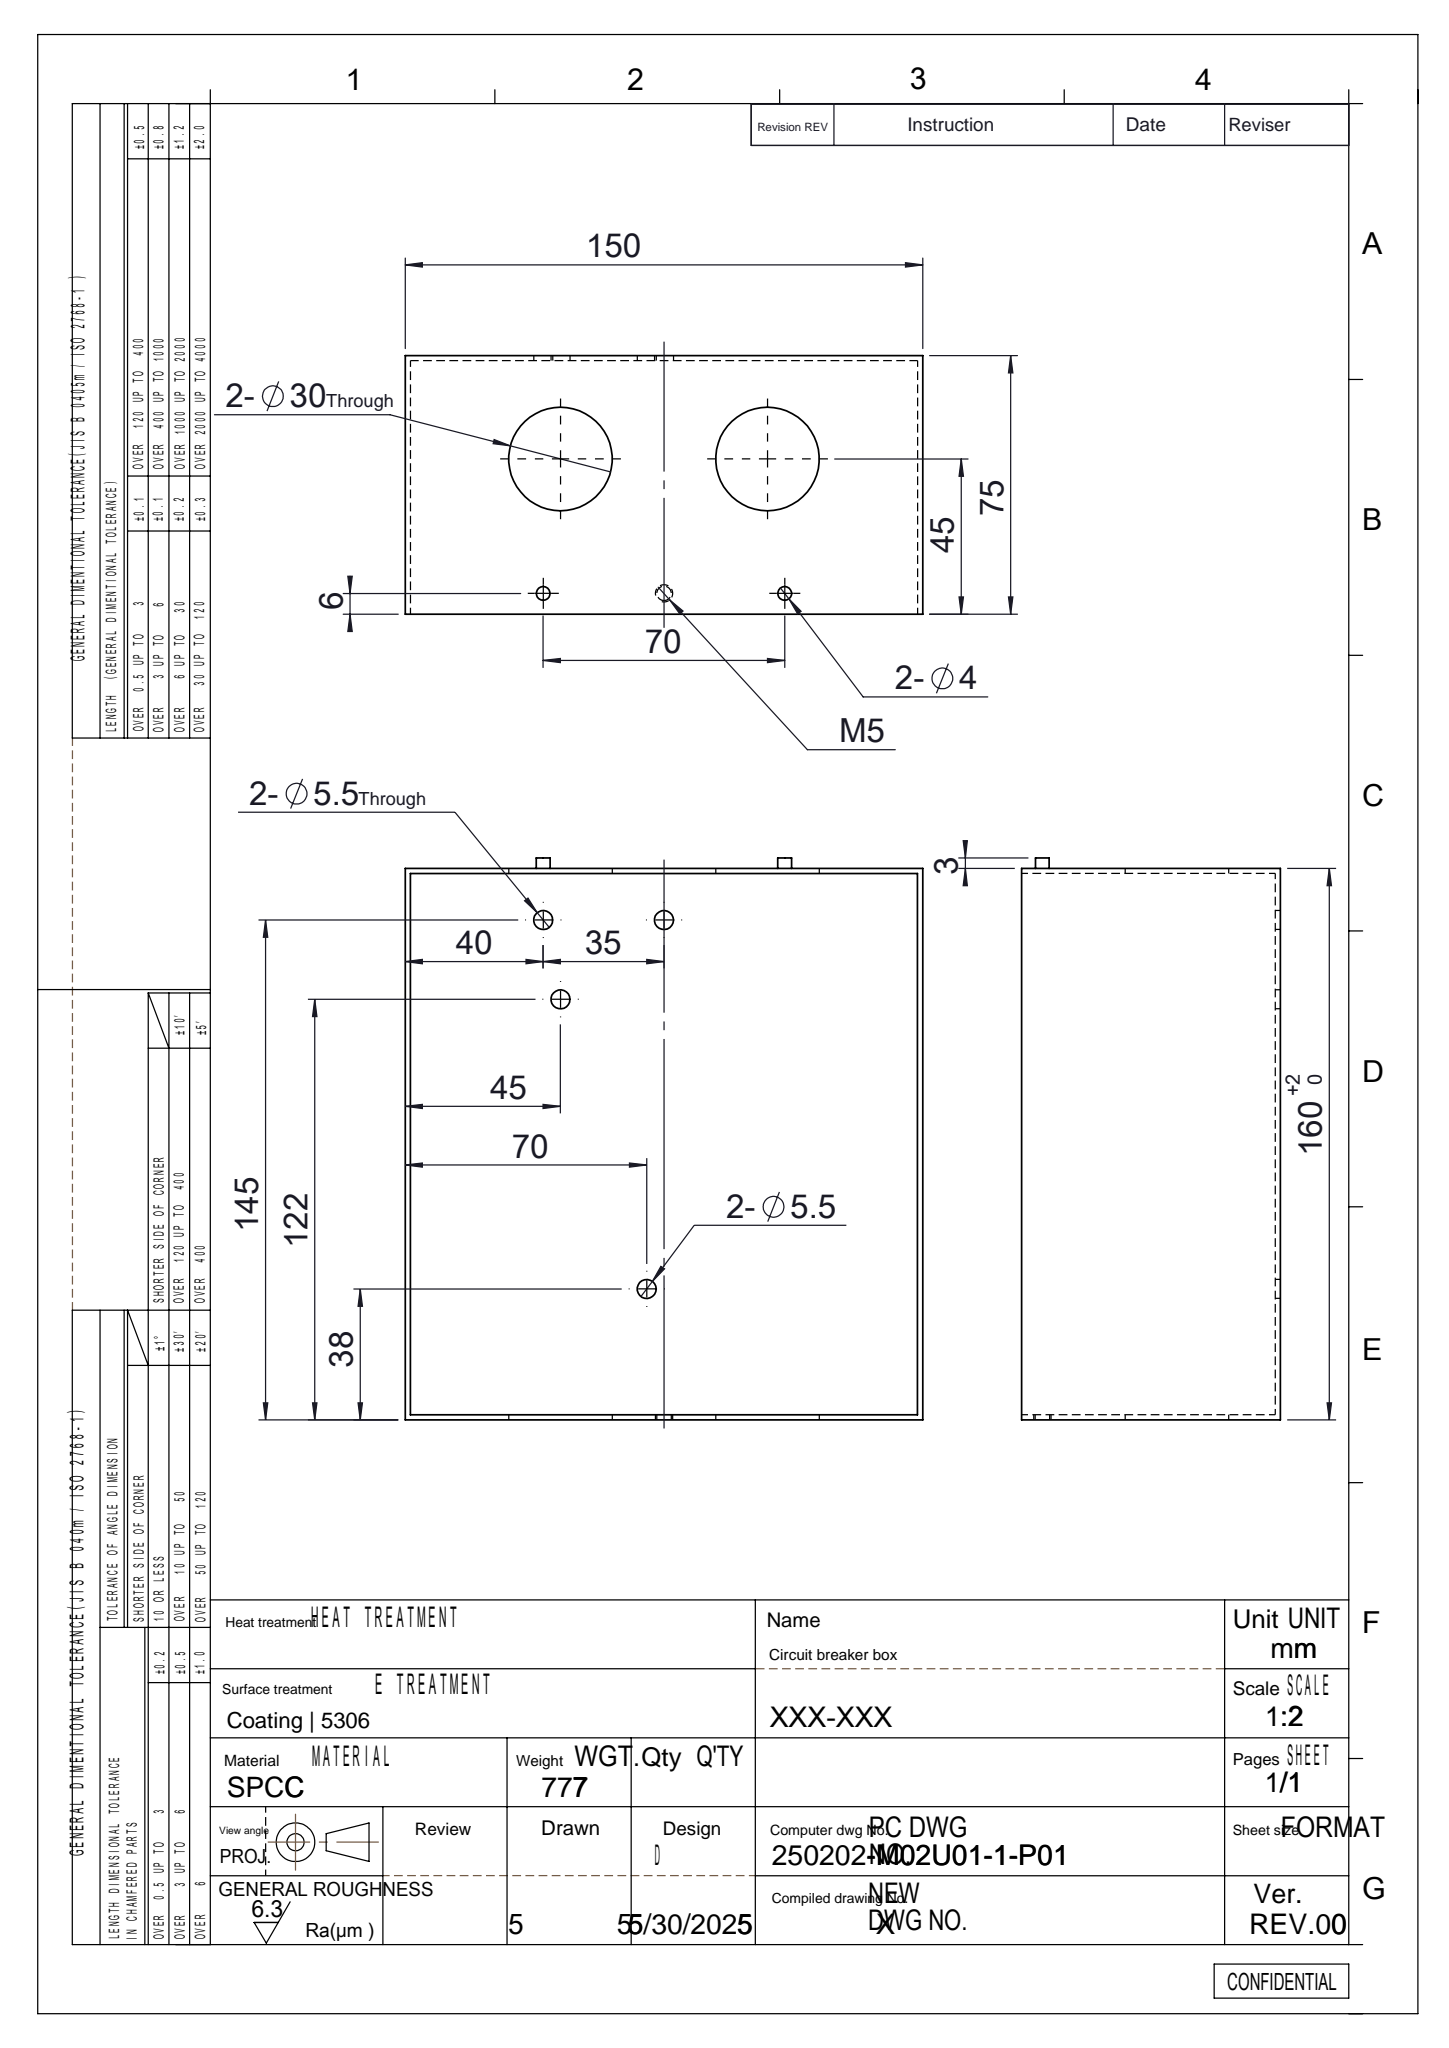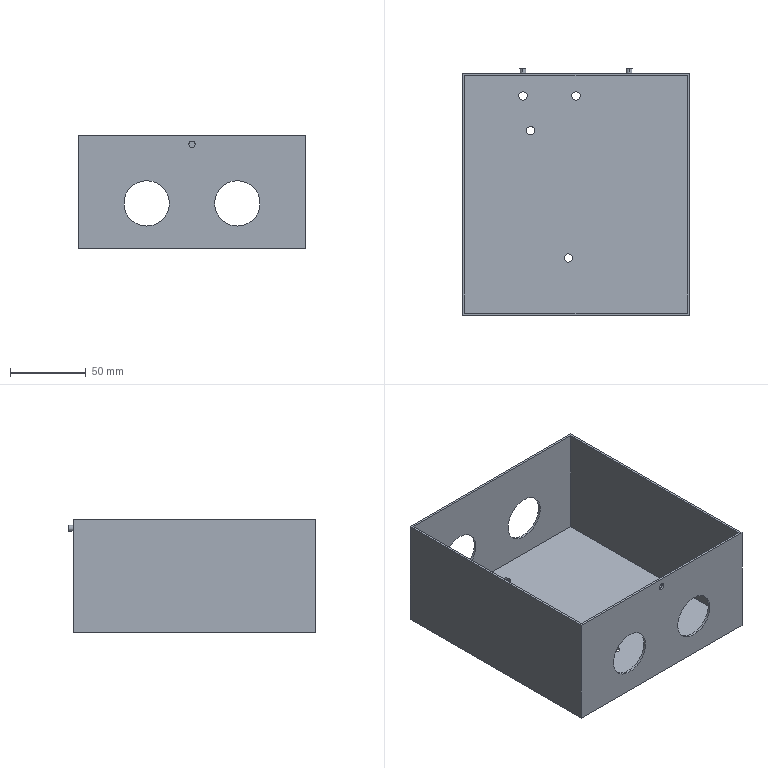Part | SolidWorks | features HoleWzd 3, ICE 2, Extrusion 1, Shell 1 | 1 solid | 35 faces | box 150 x 163 x 75 mm | volume 99364 mm3 | cylinder 22 | plane 13 | commonest cylinder face diameters 5.5 x8 30 x8 4 x4 4.2 x2